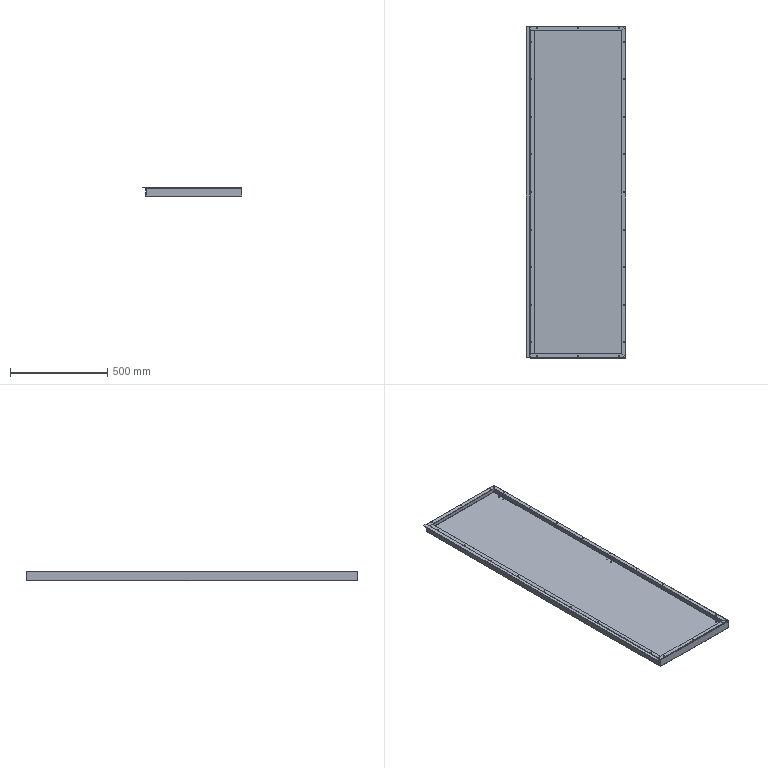Part | SolidWorks | 2 solids | 136 faces | box 512 x 1703 x 48 mm | volume 2850852 mm3 | cylinder 76 | plane 48 | spline 12 | commonest cylinder face diameters 5 x60 1.473 x8 6.473 x8